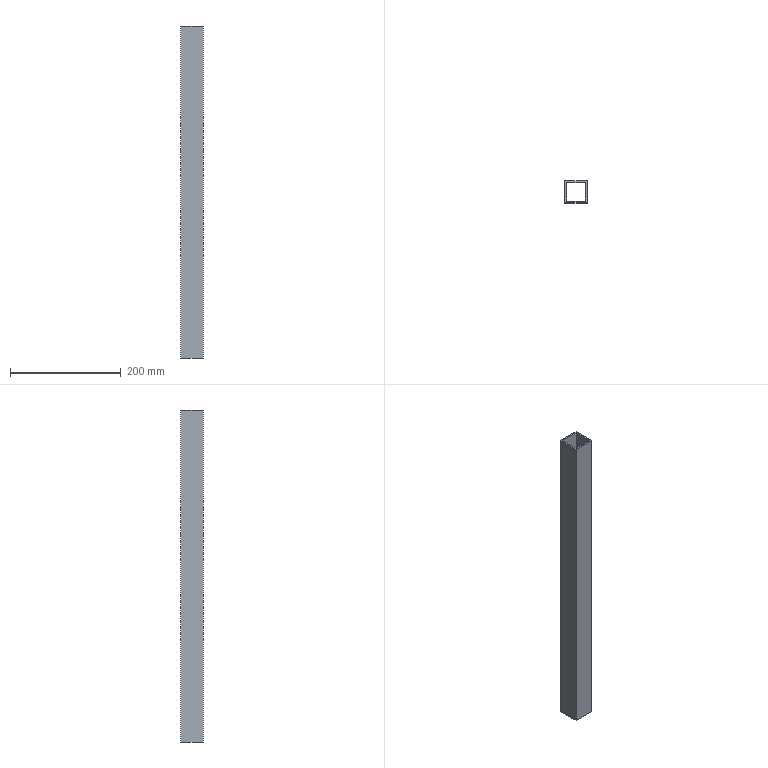Part | STEP file | BCC3 H18_5 | 1 solid | 10 faces | box 40 x 40 x 600 mm | volume 266400 mm3 | plane 10
STEP:
#1=CARTESIAN_POINT('',(0.,0.,0.));
#2=DIRECTION('',(0.,0.,1.));
#3=DIRECTION('',(1.,0.,0.));
#4=AXIS2_PLACEMENT_3D('',#1,#2,#3);
#5=CARTESIAN_POINT('',(-20.,20.,300.));
#6=VERTEX_POINT('',#5);
#7=CARTESIAN_POINT('',(-20.,-20.,300.));
#8=VERTEX_POINT('',#7);
#9=CARTESIAN_POINT('',(-20.,20.,300.));
#10=DIRECTION('',(0.,-1.,0.));
#11=VECTOR('',#10,1.);
#12=LINE('',#9,#11);
#13=CARTESIAN_POINT('',(0.,0.,300.));
#14=DIRECTION('',(0.,0.,1.));
#15=DIRECTION('',(1.,0.,0.));
#16=AXIS2_PLACEMENT_3D('',#13,#14,#15);
#17=PLANE('',#16);
#18=CARTESIAN_POINT('',(-20.,20.));
#19=DIRECTION('',(0.,-1.));
#20=VECTOR('',#19,1.);
#21=LINE('',#18,#20);
#22=(GEOMETRIC_REPRESENTATION_CONTEXT(2)PARAMETRIC_REPRESENTATION_CONTEXT()REPRESENTATION_CONTEXT('',''));
#23=DEFINITIONAL_REPRESENTATION('',(#21),#22);
#24=PCURVE('',#17,#23);
#25=CARTESIAN_POINT('',(-20.,20.,300.));
#26=DIRECTION('',(1.,0.,0.));
#27=DIRECTION('',(0.,1.,0.));
#28=AXIS2_PLACEMENT_3D('',#25,#26,#27);
#29=PLANE('',#28);
#30=CARTESIAN_POINT('',(0.,0.));
#31=DIRECTION('',(-1.,0.));
#32=VECTOR('',#31,1.);
#33=LINE('',#30,#32);
#34=(GEOMETRIC_REPRESENTATION_CONTEXT(2)PARAMETRIC_REPRESENTATION_CONTEXT()REPRESENTATION_CONTEXT('',''));
#35=DEFINITIONAL_REPRESENTATION('',(#33),#34);
#36=PCURVE('',#29,#35);
#37=SURFACE_CURVE('',#12,(#24,#36),.PCURVE_S1.);
#38=EDGE_CURVE('',#6,#8,#37,.T.);
#39=ORIENTED_EDGE('',*,*,#38,.T.);
#40=CARTESIAN_POINT('',(20.,-20.,300.));
#41=VERTEX_POINT('',#40);
#42=CARTESIAN_POINT('',(-20.,-20.,300.));
#43=DIRECTION('',(1.,0.,0.));
#44=VECTOR('',#43,1.);
#45=LINE('',#42,#44);
#46=CARTESIAN_POINT('',(-20.,-20.));
#47=DIRECTION('',(1.,0.));
#48=VECTOR('',#47,1.);
#49=LINE('',#46,#48);
#50=(GEOMETRIC_REPRESENTATION_CONTEXT(2)PARAMETRIC_REPRESENTATION_CONTEXT()REPRESENTATION_CONTEXT('',''));
#51=DEFINITIONAL_REPRESENTATION('',(#49),#50);
#52=PCURVE('',#17,#51);
#53=CARTESIAN_POINT('',(-20.,-20.,300.));
#54=DIRECTION('',(0.,1.,0.));
#55=DIRECTION('',(0.,0.,1.));
#56=AXIS2_PLACEMENT_3D('',#53,#54,#55);
#57=PLANE('',#56);
#58=CARTESIAN_POINT('',(0.,0.));
#59=DIRECTION('',(0.,1.));
#60=VECTOR('',#59,1.);
#61=LINE('',#58,#60);
#62=(GEOMETRIC_REPRESENTATION_CONTEXT(2)PARAMETRIC_REPRESENTATION_CONTEXT()REPRESENTATION_CONTEXT('',''));
#63=DEFINITIONAL_REPRESENTATION('',(#61),#62);
#64=PCURVE('',#57,#63);
#65=SURFACE_CURVE('',#45,(#52,#64),.PCURVE_S1.);
#66=EDGE_CURVE('',#8,#41,#65,.T.);
#67=ORIENTED_EDGE('',*,*,#66,.T.);
#68=CARTESIAN_POINT('',(20.,20.,300.));
#69=VERTEX_POINT('',#68);
#70=CARTESIAN_POINT('',(20.,20.,300.));
#71=DIRECTION('',(0.,1.,0.));
#72=VECTOR('',#71,1.);
#73=LINE('',#70,#72);
#74=CARTESIAN_POINT('',(20.,20.));
#75=DIRECTION('',(0.,1.));
#76=VECTOR('',#75,1.);
#77=LINE('',#74,#76);
#78=(GEOMETRIC_REPRESENTATION_CONTEXT(2)PARAMETRIC_REPRESENTATION_CONTEXT()REPRESENTATION_CONTEXT('',''));
#79=DEFINITIONAL_REPRESENTATION('',(#77),#78);
#80=PCURVE('',#17,#79);
#81=CARTESIAN_POINT('',(20.,20.,300.));
#82=DIRECTION('',(-1.,0.,0.));
#83=DIRECTION('',(0.,-1.,0.));
#84=AXIS2_PLACEMENT_3D('',#81,#82,#83);
#85=PLANE('',#84);
#86=CARTESIAN_POINT('',(0.,0.));
#87=DIRECTION('',(-1.,0.));
#88=VECTOR('',#87,1.);
#89=LINE('',#86,#88);
#90=(GEOMETRIC_REPRESENTATION_CONTEXT(2)PARAMETRIC_REPRESENTATION_CONTEXT()REPRESENTATION_CONTEXT('',''));
#91=DEFINITIONAL_REPRESENTATION('',(#89),#90);
#92=PCURVE('',#85,#91);
#93=SURFACE_CURVE('',#73,(#80,#92),.PCURVE_S1.);
#94=EDGE_CURVE('',#41,#69,#93,.T.);
#95=ORIENTED_EDGE('',*,*,#94,.T.);
#96=CARTESIAN_POINT('',(-20.,20.,300.));
#97=DIRECTION('',(-1.,0.,0.));
#98=VECTOR('',#97,1.);
#99=LINE('',#96,#98);
#100=CARTESIAN_POINT('',(-20.,20.));
#101=DIRECTION('',(-1.,0.));
#102=VECTOR('',#101,1.);
#103=LINE('',#100,#102);
#104=(GEOMETRIC_REPRESENTATION_CONTEXT(2)PARAMETRIC_REPRESENTATION_CONTEXT()REPRESENTATION_CONTEXT('',''));
#105=DEFINITIONAL_REPRESENTATION('',(#103),#104);
#106=PCURVE('',#17,#105);
#107=CARTESIAN_POINT('',(-20.,20.,300.));
#108=DIRECTION('',(0.,-1.,0.));
#109=DIRECTION('',(0.,0.,-1.));
#110=AXIS2_PLACEMENT_3D('',#107,#108,#109);
#111=PLANE('',#110);
#112=CARTESIAN_POINT('',(0.,0.));
#113=DIRECTION('',(0.,-1.));
#114=VECTOR('',#113,1.);
#115=LINE('',#112,#114);
#116=(GEOMETRIC_REPRESENTATION_CONTEXT(2)PARAMETRIC_REPRESENTATION_CONTEXT()REPRESENTATION_CONTEXT('',''));
#117=DEFINITIONAL_REPRESENTATION('',(#115),#116);
#118=PCURVE('',#111,#117);
#119=SURFACE_CURVE('',#99,(#106,#118),.PCURVE_S1.);
#120=EDGE_CURVE('',#69,#6,#119,.T.);
#121=ORIENTED_EDGE('',*,*,#120,.T.);
#122=EDGE_LOOP('',(#39,#67,#95,#121));
#123=FACE_BOUND('',#122,.T.);
#124=CARTESIAN_POINT('',(-17.,-17.,300.));
#125=VERTEX_POINT('',#124);
#126=CARTESIAN_POINT('',(17.,-17.,300.));
#127=VERTEX_POINT('',#126);
#128=CARTESIAN_POINT('',(-17.,-17.,300.));
#129=DIRECTION('',(1.,0.,0.));
#130=VECTOR('',#129,1.);
#131=LINE('',#128,#130);
#132=CARTESIAN_POINT('',(-17.,-17.));
#133=DIRECTION('',(1.,0.));
#134=VECTOR('',#133,1.);
#135=LINE('',#132,#134);
#136=(GEOMETRIC_REPRESENTATION_CONTEXT(2)PARAMETRIC_REPRESENTATION_CONTEXT()REPRESENTATION_CONTEXT('',''));
#137=DEFINITIONAL_REPRESENTATION('',(#135),#136);
#138=PCURVE('',#17,#137);
#139=CARTESIAN_POINT('',(-17.,-17.,300.));
#140=DIRECTION('',(0.,1.,0.));
#141=DIRECTION('',(-1.,0.,0.));
#142=AXIS2_PLACEMENT_3D('',#139,#140,#141);
#143=PLANE('',#142);
#144=CARTESIAN_POINT('',(0.,0.));
#145=DIRECTION('',(-1.,0.));
#146=VECTOR('',#145,1.);
#147=LINE('',#144,#146);
#148=(GEOMETRIC_REPRESENTATION_CONTEXT(2)PARAMETRIC_REPRESENTATION_CONTEXT()REPRESENTATION_CONTEXT('',''));
#149=DEFINITIONAL_REPRESENTATION('',(#147),#148);
#150=PCURVE('',#143,#149);
#151=SURFACE_CURVE('',#131,(#138,#150),.PCURVE_S1.);
#152=EDGE_CURVE('',#125,#127,#151,.T.);
#153=ORIENTED_EDGE('',*,*,#152,.F.);
#154=CARTESIAN_POINT('',(-17.,17.,300.));
#155=VERTEX_POINT('',#154);
#156=CARTESIAN_POINT('',(-17.,17.,300.));
#157=DIRECTION('',(0.,-1.,0.));
#158=VECTOR('',#157,1.);
#159=LINE('',#156,#158);
#160=CARTESIAN_POINT('',(-17.,17.));
#161=DIRECTION('',(0.,-1.));
#162=VECTOR('',#161,1.);
#163=LINE('',#160,#162);
#164=(GEOMETRIC_REPRESENTATION_CONTEXT(2)PARAMETRIC_REPRESENTATION_CONTEXT()REPRESENTATION_CONTEXT('',''));
#165=DEFINITIONAL_REPRESENTATION('',(#163),#164);
#166=PCURVE('',#17,#165);
#167=CARTESIAN_POINT('',(-17.,17.,300.));
#168=DIRECTION('',(1.,0.,0.));
#169=DIRECTION('',(0.,1.,0.));
#170=AXIS2_PLACEMENT_3D('',#167,#168,#169);
#171=PLANE('',#170);
#172=CARTESIAN_POINT('',(0.,0.));
#173=DIRECTION('',(-1.,0.));
#174=VECTOR('',#173,1.);
#175=LINE('',#172,#174);
#176=(GEOMETRIC_REPRESENTATION_CONTEXT(2)PARAMETRIC_REPRESENTATION_CONTEXT()REPRESENTATION_CONTEXT('',''));
#177=DEFINITIONAL_REPRESENTATION('',(#175),#176);
#178=PCURVE('',#171,#177);
#179=SURFACE_CURVE('',#159,(#166,#178),.PCURVE_S1.);
#180=EDGE_CURVE('',#155,#125,#179,.T.);
#181=ORIENTED_EDGE('',*,*,#180,.F.);
#182=CARTESIAN_POINT('',(17.,17.,300.));
#183=VERTEX_POINT('',#182);
#184=CARTESIAN_POINT('',(-17.,17.,300.));
#185=DIRECTION('',(-1.,0.,0.));
#186=VECTOR('',#185,1.);
#187=LINE('',#184,#186);
#188=CARTESIAN_POINT('',(-17.,17.));
#189=DIRECTION('',(-1.,0.));
#190=VECTOR('',#189,1.);
#191=LINE('',#188,#190);
#192=(GEOMETRIC_REPRESENTATION_CONTEXT(2)PARAMETRIC_REPRESENTATION_CONTEXT()REPRESENTATION_CONTEXT('',''));
#193=DEFINITIONAL_REPRESENTATION('',(#191),#192);
#194=PCURVE('',#17,#193);
#195=CARTESIAN_POINT('',(-17.,17.,300.));
#196=DIRECTION('',(0.,-1.,0.));
#197=DIRECTION('',(0.,0.,-1.));
#198=AXIS2_PLACEMENT_3D('',#195,#196,#197);
#199=PLANE('',#198);
#200=CARTESIAN_POINT('',(0.,0.));
#201=DIRECTION('',(0.,-1.));
#202=VECTOR('',#201,1.);
#203=LINE('',#200,#202);
#204=(GEOMETRIC_REPRESENTATION_CONTEXT(2)PARAMETRIC_REPRESENTATION_CONTEXT()REPRESENTATION_CONTEXT('',''));
#205=DEFINITIONAL_REPRESENTATION('',(#203),#204);
#206=PCURVE('',#199,#205);
#207=SURFACE_CURVE('',#187,(#194,#206),.PCURVE_S1.);
#208=EDGE_CURVE('',#183,#155,#207,.T.);
#209=ORIENTED_EDGE('',*,*,#208,.F.);
#210=CARTESIAN_POINT('',(17.,17.,300.));
#211=DIRECTION('',(0.,1.,0.));
#212=VECTOR('',#211,1.);
#213=LINE('',#210,#212);
#214=CARTESIAN_POINT('',(17.,17.));
#215=DIRECTION('',(0.,1.));
#216=VECTOR('',#215,1.);
#217=LINE('',#214,#216);
#218=(GEOMETRIC_REPRESENTATION_CONTEXT(2)PARAMETRIC_REPRESENTATION_CONTEXT()REPRESENTATION_CONTEXT('',''));
#219=DEFINITIONAL_REPRESENTATION('',(#217),#218);
#220=PCURVE('',#17,#219);
#221=CARTESIAN_POINT('',(17.,17.,300.));
#222=DIRECTION('',(-1.,0.,0.));
#223=DIRECTION('',(0.,-1.,0.));
#224=AXIS2_PLACEMENT_3D('',#221,#222,#223);
#225=PLANE('',#224);
#226=CARTESIAN_POINT('',(0.,0.));
#227=DIRECTION('',(-1.,0.));
#228=VECTOR('',#227,1.);
#229=LINE('',#226,#228);
#230=(GEOMETRIC_REPRESENTATION_CONTEXT(2)PARAMETRIC_REPRESENTATION_CONTEXT()REPRESENTATION_CONTEXT('',''));
#231=DEFINITIONAL_REPRESENTATION('',(#229),#230);
#232=PCURVE('',#225,#231);
#233=SURFACE_CURVE('',#213,(#220,#232),.PCURVE_S1.);
#234=EDGE_CURVE('',#127,#183,#233,.T.);
#235=ORIENTED_EDGE('',*,*,#234,.F.);
#236=EDGE_LOOP('',(#153,#181,#209,#235));
#237=FACE_BOUND('',#236,.T.);
#238=ADVANCED_FACE('',(#123,#237),#17,.T.);
#239=CARTESIAN_POINT('',(-20.,20.,-300.));
#240=VERTEX_POINT('',#239);
#241=CARTESIAN_POINT('',(-20.,-20.,-300.));
#242=VERTEX_POINT('',#241);
#243=CARTESIAN_POINT('',(-20.,20.,-300.));
#244=DIRECTION('',(0.,-1.,0.));
#245=VECTOR('',#244,1.);
#246=LINE('',#243,#245);
#247=CARTESIAN_POINT('',(0.,0.,-300.));
#248=DIRECTION('',(0.,0.,1.));
#249=DIRECTION('',(1.,0.,0.));
#250=AXIS2_PLACEMENT_3D('',#247,#248,#249);
#251=PLANE('',#250);
#252=CARTESIAN_POINT('',(-20.,20.));
#253=DIRECTION('',(0.,-1.));
#254=VECTOR('',#253,1.);
#255=LINE('',#252,#254);
#256=(GEOMETRIC_REPRESENTATION_CONTEXT(2)PARAMETRIC_REPRESENTATION_CONTEXT()REPRESENTATION_CONTEXT('',''));
#257=DEFINITIONAL_REPRESENTATION('',(#255),#256);
#258=PCURVE('',#251,#257);
#259=CARTESIAN_POINT('',(0.,-600.));
#260=DIRECTION('',(-1.,0.));
#261=VECTOR('',#260,1.);
#262=LINE('',#259,#261);
#263=(GEOMETRIC_REPRESENTATION_CONTEXT(2)PARAMETRIC_REPRESENTATION_CONTEXT()REPRESENTATION_CONTEXT('',''));
#264=DEFINITIONAL_REPRESENTATION('',(#262),#263);
#265=PCURVE('',#29,#264);
#266=SURFACE_CURVE('',#246,(#258,#265),.PCURVE_S1.);
#267=EDGE_CURVE('',#240,#242,#266,.T.);
#268=ORIENTED_EDGE('',*,*,#267,.F.);
#269=CARTESIAN_POINT('',(20.,20.,-300.));
#270=VERTEX_POINT('',#269);
#271=CARTESIAN_POINT('',(-20.,20.,-300.));
#272=DIRECTION('',(-1.,0.,0.));
#273=VECTOR('',#272,1.);
#274=LINE('',#271,#273);
#275=CARTESIAN_POINT('',(-20.,20.));
#276=DIRECTION('',(-1.,0.));
#277=VECTOR('',#276,1.);
#278=LINE('',#275,#277);
#279=(GEOMETRIC_REPRESENTATION_CONTEXT(2)PARAMETRIC_REPRESENTATION_CONTEXT()REPRESENTATION_CONTEXT('',''));
#280=DEFINITIONAL_REPRESENTATION('',(#278),#279);
#281=PCURVE('',#251,#280);
#282=CARTESIAN_POINT('',(600.,0.));
#283=DIRECTION('',(0.,-1.));
#284=VECTOR('',#283,1.);
#285=LINE('',#282,#284);
#286=(GEOMETRIC_REPRESENTATION_CONTEXT(2)PARAMETRIC_REPRESENTATION_CONTEXT()REPRESENTATION_CONTEXT('',''));
#287=DEFINITIONAL_REPRESENTATION('',(#285),#286);
#288=PCURVE('',#111,#287);
#289=SURFACE_CURVE('',#274,(#281,#288),.PCURVE_S1.);
#290=EDGE_CURVE('',#270,#240,#289,.T.);
#291=ORIENTED_EDGE('',*,*,#290,.F.);
#292=CARTESIAN_POINT('',(20.,-20.,-300.));
#293=VERTEX_POINT('',#292);
#294=CARTESIAN_POINT('',(20.,20.,-300.));
#295=DIRECTION('',(0.,1.,0.));
#296=VECTOR('',#295,1.);
#297=LINE('',#294,#296);
#298=CARTESIAN_POINT('',(20.,20.));
#299=DIRECTION('',(0.,1.));
#300=VECTOR('',#299,1.);
#301=LINE('',#298,#300);
#302=(GEOMETRIC_REPRESENTATION_CONTEXT(2)PARAMETRIC_REPRESENTATION_CONTEXT()REPRESENTATION_CONTEXT('',''));
#303=DEFINITIONAL_REPRESENTATION('',(#301),#302);
#304=PCURVE('',#251,#303);
#305=CARTESIAN_POINT('',(0.,-600.));
#306=DIRECTION('',(-1.,0.));
#307=VECTOR('',#306,1.);
#308=LINE('',#305,#307);
#309=(GEOMETRIC_REPRESENTATION_CONTEXT(2)PARAMETRIC_REPRESENTATION_CONTEXT()REPRESENTATION_CONTEXT('',''));
#310=DEFINITIONAL_REPRESENTATION('',(#308),#309);
#311=PCURVE('',#85,#310);
#312=SURFACE_CURVE('',#297,(#304,#311),.PCURVE_S1.);
#313=EDGE_CURVE('',#293,#270,#312,.T.);
#314=ORIENTED_EDGE('',*,*,#313,.F.);
#315=CARTESIAN_POINT('',(-20.,-20.,-300.));
#316=DIRECTION('',(1.,0.,0.));
#317=VECTOR('',#316,1.);
#318=LINE('',#315,#317);
#319=CARTESIAN_POINT('',(-20.,-20.));
#320=DIRECTION('',(1.,0.));
#321=VECTOR('',#320,1.);
#322=LINE('',#319,#321);
#323=(GEOMETRIC_REPRESENTATION_CONTEXT(2)PARAMETRIC_REPRESENTATION_CONTEXT()REPRESENTATION_CONTEXT('',''));
#324=DEFINITIONAL_REPRESENTATION('',(#322),#323);
#325=PCURVE('',#251,#324);
#326=CARTESIAN_POINT('',(-600.,0.));
#327=DIRECTION('',(0.,1.));
#328=VECTOR('',#327,1.);
#329=LINE('',#326,#328);
#330=(GEOMETRIC_REPRESENTATION_CONTEXT(2)PARAMETRIC_REPRESENTATION_CONTEXT()REPRESENTATION_CONTEXT('',''));
#331=DEFINITIONAL_REPRESENTATION('',(#329),#330);
#332=PCURVE('',#57,#331);
#333=SURFACE_CURVE('',#318,(#325,#332),.PCURVE_S1.);
#334=EDGE_CURVE('',#242,#293,#333,.T.);
#335=ORIENTED_EDGE('',*,*,#334,.F.);
#336=EDGE_LOOP('',(#268,#291,#314,#335));
#337=FACE_BOUND('',#336,.T.);
#338=CARTESIAN_POINT('',(-17.,17.,-300.));
#339=VERTEX_POINT('',#338);
#340=CARTESIAN_POINT('',(-17.,-17.,-300.));
#341=VERTEX_POINT('',#340);
#342=CARTESIAN_POINT('',(-17.,17.,-300.));
#343=DIRECTION('',(0.,-1.,0.));
#344=VECTOR('',#343,1.);
#345=LINE('',#342,#344);
#346=CARTESIAN_POINT('',(-17.,17.));
#347=DIRECTION('',(0.,-1.));
#348=VECTOR('',#347,1.);
#349=LINE('',#346,#348);
#350=(GEOMETRIC_REPRESENTATION_CONTEXT(2)PARAMETRIC_REPRESENTATION_CONTEXT()REPRESENTATION_CONTEXT('',''));
#351=DEFINITIONAL_REPRESENTATION('',(#349),#350);
#352=PCURVE('',#251,#351);
#353=CARTESIAN_POINT('',(0.,-600.));
#354=DIRECTION('',(-1.,0.));
#355=VECTOR('',#354,1.);
#356=LINE('',#353,#355);
#357=(GEOMETRIC_REPRESENTATION_CONTEXT(2)PARAMETRIC_REPRESENTATION_CONTEXT()REPRESENTATION_CONTEXT('',''));
#358=DEFINITIONAL_REPRESENTATION('',(#356),#357);
#359=PCURVE('',#171,#358);
#360=SURFACE_CURVE('',#345,(#352,#359),.PCURVE_S1.);
#361=EDGE_CURVE('',#339,#341,#360,.T.);
#362=ORIENTED_EDGE('',*,*,#361,.T.);
#363=CARTESIAN_POINT('',(17.,-17.,-300.));
#364=VERTEX_POINT('',#363);
#365=CARTESIAN_POINT('',(-17.,-17.,-300.));
#366=DIRECTION('',(1.,0.,0.));
#367=VECTOR('',#366,1.);
#368=LINE('',#365,#367);
#369=CARTESIAN_POINT('',(-17.,-17.));
#370=DIRECTION('',(1.,0.));
#371=VECTOR('',#370,1.);
#372=LINE('',#369,#371);
#373=(GEOMETRIC_REPRESENTATION_CONTEXT(2)PARAMETRIC_REPRESENTATION_CONTEXT()REPRESENTATION_CONTEXT('',''));
#374=DEFINITIONAL_REPRESENTATION('',(#372),#373);
#375=PCURVE('',#251,#374);
#376=CARTESIAN_POINT('',(0.,-600.));
#377=DIRECTION('',(-1.,0.));
#378=VECTOR('',#377,1.);
#379=LINE('',#376,#378);
#380=(GEOMETRIC_REPRESENTATION_CONTEXT(2)PARAMETRIC_REPRESENTATION_CONTEXT()REPRESENTATION_CONTEXT('',''));
#381=DEFINITIONAL_REPRESENTATION('',(#379),#380);
#382=PCURVE('',#143,#381);
#383=SURFACE_CURVE('',#368,(#375,#382),.PCURVE_S1.);
#384=EDGE_CURVE('',#341,#364,#383,.T.);
#385=ORIENTED_EDGE('',*,*,#384,.T.);
#386=CARTESIAN_POINT('',(17.,17.,-300.));
#387=VERTEX_POINT('',#386);
#388=CARTESIAN_POINT('',(17.,17.,-300.));
#389=DIRECTION('',(0.,1.,0.));
#390=VECTOR('',#389,1.);
#391=LINE('',#388,#390);
#392=CARTESIAN_POINT('',(17.,17.));
#393=DIRECTION('',(0.,1.));
#394=VECTOR('',#393,1.);
#395=LINE('',#392,#394);
#396=(GEOMETRIC_REPRESENTATION_CONTEXT(2)PARAMETRIC_REPRESENTATION_CONTEXT()REPRESENTATION_CONTEXT('',''));
#397=DEFINITIONAL_REPRESENTATION('',(#395),#396);
#398=PCURVE('',#251,#397);
#399=CARTESIAN_POINT('',(0.,-600.));
#400=DIRECTION('',(-1.,0.));
#401=VECTOR('',#400,1.);
#402=LINE('',#399,#401);
#403=(GEOMETRIC_REPRESENTATION_CONTEXT(2)PARAMETRIC_REPRESENTATION_CONTEXT()REPRESENTATION_CONTEXT('',''));
#404=DEFINITIONAL_REPRESENTATION('',(#402),#403);
#405=PCURVE('',#225,#404);
#406=SURFACE_CURVE('',#391,(#398,#405),.PCURVE_S1.);
#407=EDGE_CURVE('',#364,#387,#406,.T.);
#408=ORIENTED_EDGE('',*,*,#407,.T.);
#409=CARTESIAN_POINT('',(-17.,17.,-300.));
#410=DIRECTION('',(-1.,0.,0.));
#411=VECTOR('',#410,1.);
#412=LINE('',#409,#411);
#413=CARTESIAN_POINT('',(-17.,17.));
#414=DIRECTION('',(-1.,0.));
#415=VECTOR('',#414,1.);
#416=LINE('',#413,#415);
#417=(GEOMETRIC_REPRESENTATION_CONTEXT(2)PARAMETRIC_REPRESENTATION_CONTEXT()REPRESENTATION_CONTEXT('',''));
#418=DEFINITIONAL_REPRESENTATION('',(#416),#417);
#419=PCURVE('',#251,#418);
#420=CARTESIAN_POINT('',(600.,0.));
#421=DIRECTION('',(0.,-1.));
#422=VECTOR('',#421,1.);
#423=LINE('',#420,#422);
#424=(GEOMETRIC_REPRESENTATION_CONTEXT(2)PARAMETRIC_REPRESENTATION_CONTEXT()REPRESENTATION_CONTEXT('',''));
#425=DEFINITIONAL_REPRESENTATION('',(#423),#424);
#426=PCURVE('',#199,#425);
#427=SURFACE_CURVE('',#412,(#419,#426),.PCURVE_S1.);
#428=EDGE_CURVE('',#387,#339,#427,.T.);
#429=ORIENTED_EDGE('',*,*,#428,.T.);
#430=EDGE_LOOP('',(#362,#385,#408,#429));
#431=FACE_BOUND('',#430,.T.);
#432=ADVANCED_FACE('',(#337,#431),#251,.F.);
#433=ORIENTED_EDGE('',*,*,#267,.T.);
#434=CARTESIAN_POINT('',(-20.,-20.,300.));
#435=DIRECTION('',(0.,0.,-1.));
#436=VECTOR('',#435,1.);
#437=LINE('',#434,#436);
#438=CARTESIAN_POINT('',(-40.,0.));
#439=DIRECTION('',(0.,-1.));
#440=VECTOR('',#439,1.);
#441=LINE('',#438,#440);
#442=(GEOMETRIC_REPRESENTATION_CONTEXT(2)PARAMETRIC_REPRESENTATION_CONTEXT()REPRESENTATION_CONTEXT('',''));
#443=DEFINITIONAL_REPRESENTATION('',(#441),#442);
#444=PCURVE('',#29,#443);
#445=CARTESIAN_POINT('',(0.,0.));
#446=DIRECTION('',(-1.,0.));
#447=VECTOR('',#446,1.);
#448=LINE('',#445,#447);
#449=(GEOMETRIC_REPRESENTATION_CONTEXT(2)PARAMETRIC_REPRESENTATION_CONTEXT()REPRESENTATION_CONTEXT('',''));
#450=DEFINITIONAL_REPRESENTATION('',(#448),#449);
#451=PCURVE('',#57,#450);
#452=SURFACE_CURVE('',#437,(#444,#451),.PCURVE_S1.);
#453=EDGE_CURVE('',#8,#242,#452,.T.);
#454=ORIENTED_EDGE('',*,*,#453,.F.);
#455=ORIENTED_EDGE('',*,*,#38,.F.);
#456=CARTESIAN_POINT('',(-20.,20.,300.));
#457=DIRECTION('',(0.,0.,-1.));
#458=VECTOR('',#457,1.);
#459=LINE('',#456,#458);
#460=CARTESIAN_POINT('',(0.,0.));
#461=DIRECTION('',(0.,-1.));
#462=VECTOR('',#461,1.);
#463=LINE('',#460,#462);
#464=(GEOMETRIC_REPRESENTATION_CONTEXT(2)PARAMETRIC_REPRESENTATION_CONTEXT()REPRESENTATION_CONTEXT('',''));
#465=DEFINITIONAL_REPRESENTATION('',(#463),#464);
#466=PCURVE('',#29,#465);
#467=CARTESIAN_POINT('',(0.,0.));
#468=DIRECTION('',(1.,0.));
#469=VECTOR('',#468,1.);
#470=LINE('',#467,#469);
#471=(GEOMETRIC_REPRESENTATION_CONTEXT(2)PARAMETRIC_REPRESENTATION_CONTEXT()REPRESENTATION_CONTEXT('',''));
#472=DEFINITIONAL_REPRESENTATION('',(#470),#471);
#473=PCURVE('',#111,#472);
#474=SURFACE_CURVE('',#459,(#466,#473),.PCURVE_S1.);
#475=EDGE_CURVE('',#6,#240,#474,.T.);
#476=ORIENTED_EDGE('',*,*,#475,.T.);
#477=EDGE_LOOP('',(#433,#454,#455,#476));
#478=FACE_BOUND('',#477,.T.);
#479=ADVANCED_FACE('',(#478),#29,.F.);
#480=ORIENTED_EDGE('',*,*,#334,.T.);
#481=CARTESIAN_POINT('',(20.,-20.,300.));
#482=DIRECTION('',(0.,0.,-1.));
#483=VECTOR('',#482,1.);
#484=LINE('',#481,#483);
#485=CARTESIAN_POINT('',(0.,40.));
#486=DIRECTION('',(-1.,0.));
#487=VECTOR('',#486,1.);
#488=LINE('',#485,#487);
#489=(GEOMETRIC_REPRESENTATION_CONTEXT(2)PARAMETRIC_REPRESENTATION_CONTEXT()REPRESENTATION_CONTEXT('',''));
#490=DEFINITIONAL_REPRESENTATION('',(#488),#489);
#491=PCURVE('',#57,#490);
#492=CARTESIAN_POINT('',(40.,0.));
#493=DIRECTION('',(0.,-1.));
#494=VECTOR('',#493,1.);
#495=LINE('',#492,#494);
#496=(GEOMETRIC_REPRESENTATION_CONTEXT(2)PARAMETRIC_REPRESENTATION_CONTEXT()REPRESENTATION_CONTEXT('',''));
#497=DEFINITIONAL_REPRESENTATION('',(#495),#496);
#498=PCURVE('',#85,#497);
#499=SURFACE_CURVE('',#484,(#491,#498),.PCURVE_S1.);
#500=EDGE_CURVE('',#41,#293,#499,.T.);
#501=ORIENTED_EDGE('',*,*,#500,.F.);
#502=ORIENTED_EDGE('',*,*,#66,.F.);
#503=ORIENTED_EDGE('',*,*,#453,.T.);
#504=EDGE_LOOP('',(#480,#501,#502,#503));
#505=FACE_BOUND('',#504,.T.);
#506=ADVANCED_FACE('',(#505),#57,.F.);
#507=ORIENTED_EDGE('',*,*,#313,.T.);
#508=CARTESIAN_POINT('',(20.,20.,300.));
#509=DIRECTION('',(0.,0.,-1.));
#510=VECTOR('',#509,1.);
#511=LINE('',#508,#510);
#512=CARTESIAN_POINT('',(0.,0.));
#513=DIRECTION('',(0.,-1.));
#514=VECTOR('',#513,1.);
#515=LINE('',#512,#514);
#516=(GEOMETRIC_REPRESENTATION_CONTEXT(2)PARAMETRIC_REPRESENTATION_CONTEXT()REPRESENTATION_CONTEXT('',''));
#517=DEFINITIONAL_REPRESENTATION('',(#515),#516);
#518=PCURVE('',#85,#517);
#519=CARTESIAN_POINT('',(0.,40.));
#520=DIRECTION('',(1.,0.));
#521=VECTOR('',#520,1.);
#522=LINE('',#519,#521);
#523=(GEOMETRIC_REPRESENTATION_CONTEXT(2)PARAMETRIC_REPRESENTATION_CONTEXT()REPRESENTATION_CONTEXT('',''));
#524=DEFINITIONAL_REPRESENTATION('',(#522),#523);
#525=PCURVE('',#111,#524);
#526=SURFACE_CURVE('',#511,(#518,#525),.PCURVE_S1.);
#527=EDGE_CURVE('',#69,#270,#526,.T.);
#528=ORIENTED_EDGE('',*,*,#527,.F.);
#529=ORIENTED_EDGE('',*,*,#94,.F.);
#530=ORIENTED_EDGE('',*,*,#500,.T.);
#531=EDGE_LOOP('',(#507,#528,#529,#530));
#532=FACE_BOUND('',#531,.T.);
#533=ADVANCED_FACE('',(#532),#85,.F.);
#534=ORIENTED_EDGE('',*,*,#290,.T.);
#535=ORIENTED_EDGE('',*,*,#475,.F.);
#536=ORIENTED_EDGE('',*,*,#120,.F.);
#537=ORIENTED_EDGE('',*,*,#527,.T.);
#538=EDGE_LOOP('',(#534,#535,#536,#537));
#539=FACE_BOUND('',#538,.T.);
#540=ADVANCED_FACE('',(#539),#111,.F.);
#541=ORIENTED_EDGE('',*,*,#361,.F.);
#542=CARTESIAN_POINT('',(-17.,17.,300.));
#543=DIRECTION('',(0.,0.,-1.));
#544=VECTOR('',#543,1.);
#545=LINE('',#542,#544);
#546=CARTESIAN_POINT('',(0.,0.));
#547=DIRECTION('',(0.,-1.));
#548=VECTOR('',#547,1.);
#549=LINE('',#546,#548);
#550=(GEOMETRIC_REPRESENTATION_CONTEXT(2)PARAMETRIC_REPRESENTATION_CONTEXT()REPRESENTATION_CONTEXT('',''));
#551=DEFINITIONAL_REPRESENTATION('',(#549),#550);
#552=PCURVE('',#171,#551);
#553=CARTESIAN_POINT('',(0.,0.));
#554=DIRECTION('',(1.,0.));
#555=VECTOR('',#554,1.);
#556=LINE('',#553,#555);
#557=(GEOMETRIC_REPRESENTATION_CONTEXT(2)PARAMETRIC_REPRESENTATION_CONTEXT()REPRESENTATION_CONTEXT('',''));
#558=DEFINITIONAL_REPRESENTATION('',(#556),#557);
#559=PCURVE('',#199,#558);
#560=SURFACE_CURVE('',#545,(#552,#559),.PCURVE_S1.);
#561=EDGE_CURVE('',#155,#339,#560,.T.);
#562=ORIENTED_EDGE('',*,*,#561,.F.);
#563=ORIENTED_EDGE('',*,*,#180,.T.);
#564=CARTESIAN_POINT('',(-17.,-17.,300.));
#565=DIRECTION('',(0.,0.,-1.));
#566=VECTOR('',#565,1.);
#567=LINE('',#564,#566);
#568=CARTESIAN_POINT('',(-34.,0.));
#569=DIRECTION('',(0.,-1.));
#570=VECTOR('',#569,1.);
#571=LINE('',#568,#570);
#572=(GEOMETRIC_REPRESENTATION_CONTEXT(2)PARAMETRIC_REPRESENTATION_CONTEXT()REPRESENTATION_CONTEXT('',''));
#573=DEFINITIONAL_REPRESENTATION('',(#571),#572);
#574=PCURVE('',#171,#573);
#575=CARTESIAN_POINT('',(0.,0.));
#576=DIRECTION('',(0.,-1.));
#577=VECTOR('',#576,1.);
#578=LINE('',#575,#577);
#579=(GEOMETRIC_REPRESENTATION_CONTEXT(2)PARAMETRIC_REPRESENTATION_CONTEXT()REPRESENTATION_CONTEXT('',''));
#580=DEFINITIONAL_REPRESENTATION('',(#578),#579);
#581=PCURVE('',#143,#580);
#582=SURFACE_CURVE('',#567,(#574,#581),.PCURVE_S1.);
#583=EDGE_CURVE('',#125,#341,#582,.T.);
#584=ORIENTED_EDGE('',*,*,#583,.T.);
#585=EDGE_LOOP('',(#541,#562,#563,#584));
#586=FACE_BOUND('',#585,.T.);
#587=ADVANCED_FACE('',(#586),#171,.T.);
#588=ORIENTED_EDGE('',*,*,#384,.F.);
#589=ORIENTED_EDGE('',*,*,#583,.F.);
#590=ORIENTED_EDGE('',*,*,#152,.T.);
#591=CARTESIAN_POINT('',(17.,-17.,300.));
#592=DIRECTION('',(0.,0.,-1.));
#593=VECTOR('',#592,1.);
#594=LINE('',#591,#593);
#595=CARTESIAN_POINT('',(-34.,0.));
#596=DIRECTION('',(0.,-1.));
#597=VECTOR('',#596,1.);
#598=LINE('',#595,#597);
#599=(GEOMETRIC_REPRESENTATION_CONTEXT(2)PARAMETRIC_REPRESENTATION_CONTEXT()REPRESENTATION_CONTEXT('',''));
#600=DEFINITIONAL_REPRESENTATION('',(#598),#599);
#601=PCURVE('',#143,#600);
#602=CARTESIAN_POINT('',(34.,0.));
#603=DIRECTION('',(0.,-1.));
#604=VECTOR('',#603,1.);
#605=LINE('',#602,#604);
#606=(GEOMETRIC_REPRESENTATION_CONTEXT(2)PARAMETRIC_REPRESENTATION_CONTEXT()REPRESENTATION_CONTEXT('',''));
#607=DEFINITIONAL_REPRESENTATION('',(#605),#606);
#608=PCURVE('',#225,#607);
#609=SURFACE_CURVE('',#594,(#601,#608),.PCURVE_S1.);
#610=EDGE_CURVE('',#127,#364,#609,.T.);
#611=ORIENTED_EDGE('',*,*,#610,.T.);
#612=EDGE_LOOP('',(#588,#589,#590,#611));
#613=FACE_BOUND('',#612,.T.);
#614=ADVANCED_FACE('',(#613),#143,.T.);
#615=ORIENTED_EDGE('',*,*,#407,.F.);
#616=ORIENTED_EDGE('',*,*,#610,.F.);
#617=ORIENTED_EDGE('',*,*,#234,.T.);
#618=CARTESIAN_POINT('',(17.,17.,300.));
#619=DIRECTION('',(0.,0.,-1.));
#620=VECTOR('',#619,1.);
#621=LINE('',#618,#620);
#622=CARTESIAN_POINT('',(0.,0.));
#623=DIRECTION('',(0.,-1.));
#624=VECTOR('',#623,1.);
#625=LINE('',#622,#624);
#626=(GEOMETRIC_REPRESENTATION_CONTEXT(2)PARAMETRIC_REPRESENTATION_CONTEXT()REPRESENTATION_CONTEXT('',''));
#627=DEFINITIONAL_REPRESENTATION('',(#625),#626);
#628=PCURVE('',#225,#627);
#629=CARTESIAN_POINT('',(0.,34.));
#630=DIRECTION('',(1.,0.));
#631=VECTOR('',#630,1.);
#632=LINE('',#629,#631);
#633=(GEOMETRIC_REPRESENTATION_CONTEXT(2)PARAMETRIC_REPRESENTATION_CONTEXT()REPRESENTATION_CONTEXT('',''));
#634=DEFINITIONAL_REPRESENTATION('',(#632),#633);
#635=PCURVE('',#199,#634);
#636=SURFACE_CURVE('',#621,(#628,#635),.PCURVE_S1.);
#637=EDGE_CURVE('',#183,#387,#636,.T.);
#638=ORIENTED_EDGE('',*,*,#637,.T.);
#639=EDGE_LOOP('',(#615,#616,#617,#638));
#640=FACE_BOUND('',#639,.T.);
#641=ADVANCED_FACE('',(#640),#225,.T.);
#642=ORIENTED_EDGE('',*,*,#428,.F.);
#643=ORIENTED_EDGE('',*,*,#637,.F.);
#644=ORIENTED_EDGE('',*,*,#208,.T.);
#645=ORIENTED_EDGE('',*,*,#561,.T.);
#646=EDGE_LOOP('',(#642,#643,#644,#645));
#647=FACE_BOUND('',#646,.T.);
#648=ADVANCED_FACE('',(#647),#199,.T.);
#649=CLOSED_SHELL('',(#238,#432,#479,#506,#533,#540,#587,#614,#641,#648));
#650=MANIFOLD_SOLID_BREP('',#649);
#651=(LENGTH_UNIT()NAMED_UNIT(*)SI_UNIT(.MILLI.,.METRE.));
#652=UNCERTAINTY_MEASURE_WITH_UNIT(LENGTH_MEASURE(0.0000001),#651,'','');
#653=(NAMED_UNIT(*)PLANE_ANGLE_UNIT()SI_UNIT($,.RADIAN.));
#654=(NAMED_UNIT(*)SI_UNIT($,.STERADIAN.)SOLID_ANGLE_UNIT());
#655=(GEOMETRIC_REPRESENTATION_CONTEXT(3)GLOBAL_UNCERTAINTY_ASSIGNED_CONTEXT((#652))GLOBAL_UNIT_ASSIGNED_CONTEXT((#651,#653,#654))REPRESENTATION_CONTEXT('',''));
#656=ADVANCED_BREP_SHAPE_REPRESENTATION('',(#4,#650),#655);